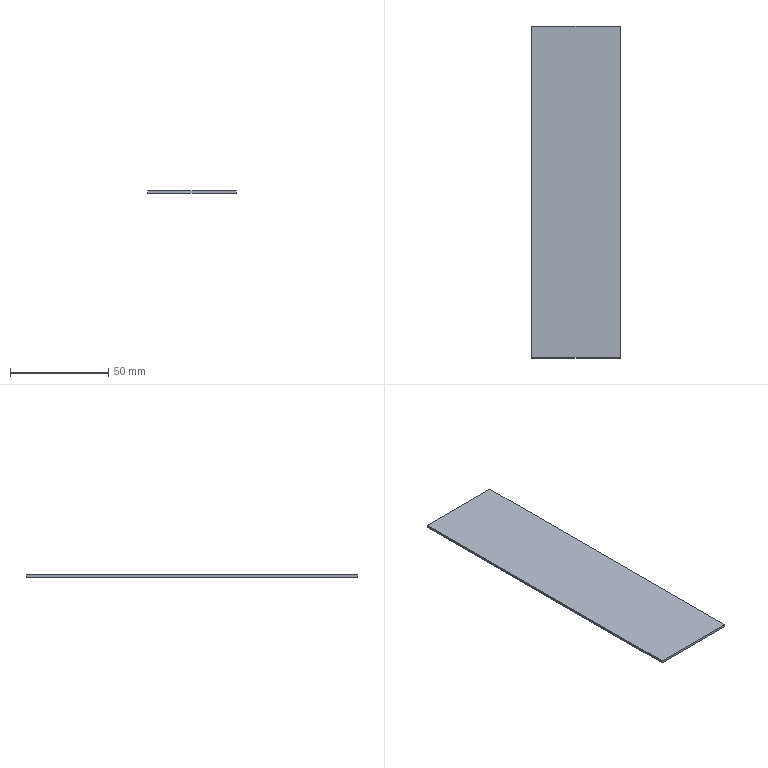Part | SolidWorks | features FlatPattern 1, SMBaseFlange 1, SheetMetal 1 | 1 solid | 6 faces | box 45 x 168.6 x 1.2 mm | volume 9104 mm3 | plane 6
STEP:
#1=CARTESIAN_POINT('',(30.,0.,0.));
#2=VERTEX_POINT('',#1);
#3=CARTESIAN_POINT('',(30.,168.6,0.));
#4=VERTEX_POINT('',#3);
#5=CARTESIAN_POINT('',(30.,168.6,0.));
#6=DIRECTION('',(0.,1.,0.));
#7=VECTOR('',#6,1000.);
#8=LINE('',#5,#7);
#9=EDGE_CURVE('',#2,#4,#8,.T.);
#10=ORIENTED_EDGE('',*,*,#9,.T.);
#11=CARTESIAN_POINT('',(30.,168.6,1.2));
#12=VERTEX_POINT('',#11);
#13=CARTESIAN_POINT('',(30.,168.6,1.2));
#14=DIRECTION('',(0.,0.,-1.));
#15=VECTOR('',#14,1000.);
#16=LINE('',#13,#15);
#17=EDGE_CURVE('',#12,#4,#16,.T.);
#18=ORIENTED_EDGE('',*,*,#17,.F.);
#19=CARTESIAN_POINT('',(30.,0.,1.2));
#20=VERTEX_POINT('',#19);
#21=CARTESIAN_POINT('',(30.,168.6,1.2));
#22=DIRECTION('',(0.,1.,0.));
#23=VECTOR('',#22,1000.);
#24=LINE('',#21,#23);
#25=EDGE_CURVE('',#20,#12,#24,.T.);
#26=ORIENTED_EDGE('',*,*,#25,.F.);
#27=CARTESIAN_POINT('',(30.,0.,1.2));
#28=DIRECTION('',(0.,0.,-1.));
#29=VECTOR('',#28,1000.);
#30=LINE('',#27,#29);
#31=EDGE_CURVE('',#20,#2,#30,.T.);
#32=ORIENTED_EDGE('',*,*,#31,.T.);
#33=EDGE_LOOP('',(#10,#18,#26,#32));
#34=FACE_OUTER_BOUND('',#33,.T.);
#35=CARTESIAN_POINT('',(30.,168.6,1.2));
#36=DIRECTION('',(-1.,0.,0.));
#37=DIRECTION('',(0.,-1.,0.));
#38=AXIS2_PLACEMENT_3D('',#35,#36,#37);
#39=PLANE('',#38);
#40=ADVANCED_FACE('',(#34),#39,.F.);
#41=CARTESIAN_POINT('',(-15.,168.6,0.));
#42=VERTEX_POINT('',#41);
#43=CARTESIAN_POINT('',(30.,168.6,0.));
#44=DIRECTION('',(-1.,0.,0.));
#45=VECTOR('',#44,1000.);
#46=LINE('',#43,#45);
#47=EDGE_CURVE('',#4,#42,#46,.T.);
#48=ORIENTED_EDGE('',*,*,#47,.T.);
#49=CARTESIAN_POINT('',(-15.,168.6,1.2));
#50=VERTEX_POINT('',#49);
#51=CARTESIAN_POINT('',(-15.,168.6,1.2));
#52=DIRECTION('',(0.,0.,-1.));
#53=VECTOR('',#52,1000.);
#54=LINE('',#51,#53);
#55=EDGE_CURVE('',#50,#42,#54,.T.);
#56=ORIENTED_EDGE('',*,*,#55,.F.);
#57=CARTESIAN_POINT('',(30.,168.6,1.2));
#58=DIRECTION('',(-1.,0.,0.));
#59=VECTOR('',#58,1000.);
#60=LINE('',#57,#59);
#61=EDGE_CURVE('',#12,#50,#60,.T.);
#62=ORIENTED_EDGE('',*,*,#61,.F.);
#63=ORIENTED_EDGE('',*,*,#17,.T.);
#64=EDGE_LOOP('',(#48,#56,#62,#63));
#65=FACE_OUTER_BOUND('',#64,.T.);
#66=CARTESIAN_POINT('',(30.,168.6,1.2));
#67=DIRECTION('',(0.,-1.,0.));
#68=DIRECTION('',(0.,0.,-1.));
#69=AXIS2_PLACEMENT_3D('',#66,#67,#68);
#70=PLANE('',#69);
#71=ADVANCED_FACE('',(#65),#70,.F.);
#72=CARTESIAN_POINT('',(-15.,0.,0.));
#73=VERTEX_POINT('',#72);
#74=CARTESIAN_POINT('',(-15.,168.6,0.));
#75=DIRECTION('',(0.,-1.,0.));
#76=VECTOR('',#75,1000.);
#77=LINE('',#74,#76);
#78=EDGE_CURVE('',#42,#73,#77,.T.);
#79=ORIENTED_EDGE('',*,*,#78,.T.);
#80=CARTESIAN_POINT('',(-15.,0.,1.2));
#81=VERTEX_POINT('',#80);
#82=CARTESIAN_POINT('',(-15.,0.,1.2));
#83=DIRECTION('',(0.,0.,-1.));
#84=VECTOR('',#83,1000.);
#85=LINE('',#82,#84);
#86=EDGE_CURVE('',#81,#73,#85,.T.);
#87=ORIENTED_EDGE('',*,*,#86,.F.);
#88=CARTESIAN_POINT('',(-15.,168.6,1.2));
#89=DIRECTION('',(0.,-1.,0.));
#90=VECTOR('',#89,1000.);
#91=LINE('',#88,#90);
#92=EDGE_CURVE('',#50,#81,#91,.T.);
#93=ORIENTED_EDGE('',*,*,#92,.F.);
#94=ORIENTED_EDGE('',*,*,#55,.T.);
#95=EDGE_LOOP('',(#79,#87,#93,#94));
#96=FACE_OUTER_BOUND('',#95,.T.);
#97=CARTESIAN_POINT('',(-15.,168.6,1.2));
#98=DIRECTION('',(1.,0.,0.));
#99=DIRECTION('',(0.,1.,0.));
#100=AXIS2_PLACEMENT_3D('',#97,#98,#99);
#101=PLANE('',#100);
#102=ADVANCED_FACE('',(#96),#101,.F.);
#103=CARTESIAN_POINT('',(30.,0.,0.));
#104=DIRECTION('',(1.,0.,0.));
#105=VECTOR('',#104,1000.);
#106=LINE('',#103,#105);
#107=EDGE_CURVE('',#73,#2,#106,.T.);
#108=ORIENTED_EDGE('',*,*,#107,.T.);
#109=ORIENTED_EDGE('',*,*,#31,.F.);
#110=CARTESIAN_POINT('',(30.,0.,1.2));
#111=DIRECTION('',(1.,0.,0.));
#112=VECTOR('',#111,1000.);
#113=LINE('',#110,#112);
#114=EDGE_CURVE('',#81,#20,#113,.T.);
#115=ORIENTED_EDGE('',*,*,#114,.F.);
#116=ORIENTED_EDGE('',*,*,#86,.T.);
#117=EDGE_LOOP('',(#108,#109,#115,#116));
#118=FACE_OUTER_BOUND('',#117,.T.);
#119=CARTESIAN_POINT('',(30.,0.,1.2));
#120=DIRECTION('',(0.,1.,0.));
#121=DIRECTION('',(0.,0.,1.));
#122=AXIS2_PLACEMENT_3D('',#119,#120,#121);
#123=PLANE('',#122);
#124=ADVANCED_FACE('',(#118),#123,.F.);
#125=ORIENTED_EDGE('',*,*,#25,.T.);
#126=ORIENTED_EDGE('',*,*,#61,.T.);
#127=ORIENTED_EDGE('',*,*,#92,.T.);
#128=ORIENTED_EDGE('',*,*,#114,.T.);
#129=EDGE_LOOP('',(#125,#126,#127,#128));
#130=FACE_OUTER_BOUND('',#129,.T.);
#131=CARTESIAN_POINT('',(30.,0.,1.2));
#132=DIRECTION('',(0.,0.,-1.));
#133=DIRECTION('',(-1.,0.,0.));
#134=AXIS2_PLACEMENT_3D('',#131,#132,#133);
#135=PLANE('',#134);
#136=ADVANCED_FACE('',(#130),#135,.F.);
#137=ORIENTED_EDGE('',*,*,#9,.F.);
#138=ORIENTED_EDGE('',*,*,#107,.F.);
#139=ORIENTED_EDGE('',*,*,#78,.F.);
#140=ORIENTED_EDGE('',*,*,#47,.F.);
#141=EDGE_LOOP('',(#137,#138,#139,#140));
#142=FACE_OUTER_BOUND('',#141,.T.);
#143=CARTESIAN_POINT('',(30.,0.,0.));
#144=DIRECTION('',(0.,0.,-1.));
#145=DIRECTION('',(-1.,0.,0.));
#146=AXIS2_PLACEMENT_3D('',#143,#144,#145);
#147=PLANE('',#146);
#148=ADVANCED_FACE('',(#142),#147,.T.);
#149=CLOSED_SHELL('',(#40,#71,#102,#124,#136,#148));
#150=MANIFOLD_SOLID_BREP('',#149);
#151=CARTESIAN_POINT('',(0.,0.,0.));
#152=DIRECTION('',(0.,0.,1.));
#153=DIRECTION('',(1.,0.,0.));
#154=AXIS2_PLACEMENT_3D('',#151,#152,#153);
#155=(LENGTH_UNIT()NAMED_UNIT(*)SI_UNIT(.MILLI.,.METRE.));
#156=UNCERTAINTY_MEASURE_WITH_UNIT(LENGTH_MEASURE(0.00001),#155,'','');
#157=(NAMED_UNIT(*)PLANE_ANGLE_UNIT()SI_UNIT($,.RADIAN.));
#158=(NAMED_UNIT(*)SI_UNIT($,.STERADIAN.)SOLID_ANGLE_UNIT());
#159=(GEOMETRIC_REPRESENTATION_CONTEXT(3)GLOBAL_UNCERTAINTY_ASSIGNED_CONTEXT((#156))GLOBAL_UNIT_ASSIGNED_CONTEXT((#155,#157,#158))REPRESENTATION_CONTEXT('',''));
#160=ADVANCED_BREP_SHAPE_REPRESENTATION('',(#150,#154),#159);